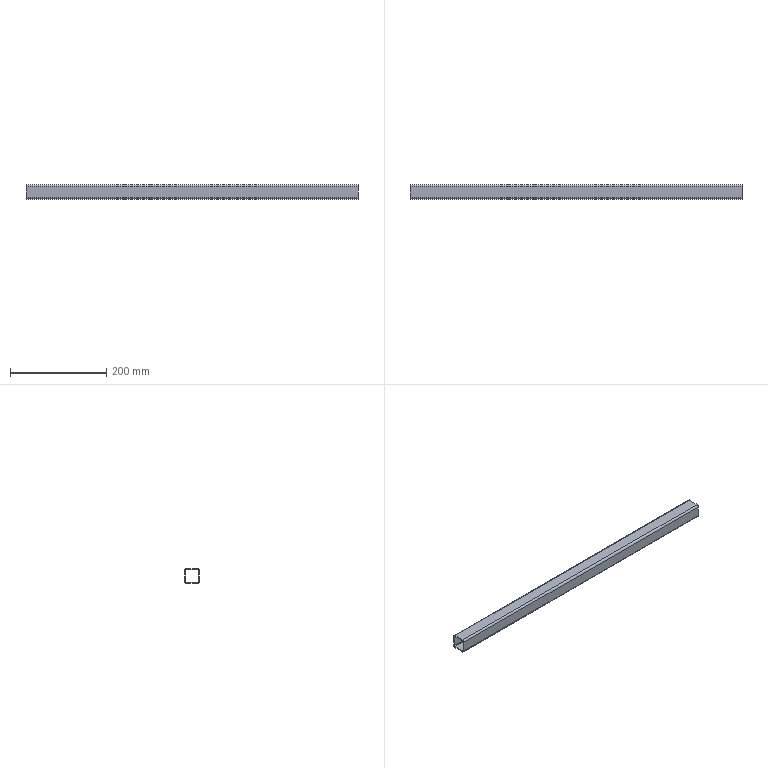Part | SolidWorks | features BaseBody 1, MoveFace 1 | 1 solid | 18 faces | box 690 x 30 x 30 mm | volume 147452 mm3 | plane 10 | cylinder 8 | commonest cylinder face diameters 4 x4 8 x4
STEP:
#1=CARTESIAN_POINT('',(-345.,-776.,31.5));
#2=VERTEX_POINT('',#1);
#3=CARTESIAN_POINT('',(-345.,-780.,27.5));
#4=VERTEX_POINT('',#3);
#5=CARTESIAN_POINT('',(-345.,-776.,27.5));
#6=DIRECTION('',(1.,0.,0.));
#7=DIRECTION('',(0.,0.,-1.));
#8=AXIS2_PLACEMENT_3D('',#5,#6,#7);
#9=CIRCLE('',#8,4.);
#10=EDGE_CURVE('',#2,#4,#9,.T.);
#11=ORIENTED_EDGE('',*,*,#10,.T.);
#12=CARTESIAN_POINT('',(345.,-780.,27.5));
#13=VERTEX_POINT('',#12);
#14=CARTESIAN_POINT('',(373.,-780.,27.5));
#15=DIRECTION('',(-1.,0.,0.));
#16=VECTOR('',#15,1000.);
#17=LINE('',#14,#16);
#18=EDGE_CURVE('',#13,#4,#17,.T.);
#19=ORIENTED_EDGE('',*,*,#18,.F.);
#20=CARTESIAN_POINT('',(345.,-776.,31.5));
#21=VERTEX_POINT('',#20);
#22=CARTESIAN_POINT('',(345.,-776.,27.5));
#23=DIRECTION('',(1.,0.,0.));
#24=DIRECTION('',(0.,0.,-1.));
#25=AXIS2_PLACEMENT_3D('',#22,#23,#24);
#26=CIRCLE('',#25,4.);
#27=EDGE_CURVE('',#21,#13,#26,.T.);
#28=ORIENTED_EDGE('',*,*,#27,.F.);
#29=CARTESIAN_POINT('',(373.,-776.,31.5));
#30=DIRECTION('',(-1.,0.,0.));
#31=VECTOR('',#30,1000.);
#32=LINE('',#29,#31);
#33=EDGE_CURVE('',#21,#2,#32,.T.);
#34=ORIENTED_EDGE('',*,*,#33,.T.);
#35=EDGE_LOOP('',(#11,#19,#28,#34));
#36=FACE_OUTER_BOUND('',#35,.T.);
#37=CARTESIAN_POINT('',(373.,-776.,27.5));
#38=DIRECTION('',(-1.,0.,0.));
#39=DIRECTION('',(0.,0.,1.));
#40=AXIS2_PLACEMENT_3D('',#37,#38,#39);
#41=CYLINDRICAL_SURFACE('',#40,4.);
#42=ADVANCED_FACE('',(#36),#41,.T.);
#43=CARTESIAN_POINT('',(-345.,-780.,5.5));
#44=VERTEX_POINT('',#43);
#45=CARTESIAN_POINT('',(-345.,-780.,27.5));
#46=DIRECTION('',(0.,0.,-1.));
#47=VECTOR('',#46,1000.);
#48=LINE('',#45,#47);
#49=EDGE_CURVE('',#4,#44,#48,.T.);
#50=ORIENTED_EDGE('',*,*,#49,.T.);
#51=CARTESIAN_POINT('',(345.,-780.,5.5));
#52=VERTEX_POINT('',#51);
#53=CARTESIAN_POINT('',(373.,-780.,5.5));
#54=DIRECTION('',(-1.,0.,0.));
#55=VECTOR('',#54,1000.);
#56=LINE('',#53,#55);
#57=EDGE_CURVE('',#52,#44,#56,.T.);
#58=ORIENTED_EDGE('',*,*,#57,.F.);
#59=CARTESIAN_POINT('',(345.,-780.,27.5));
#60=DIRECTION('',(0.,0.,-1.));
#61=VECTOR('',#60,1000.);
#62=LINE('',#59,#61);
#63=EDGE_CURVE('',#13,#52,#62,.T.);
#64=ORIENTED_EDGE('',*,*,#63,.F.);
#65=ORIENTED_EDGE('',*,*,#18,.T.);
#66=EDGE_LOOP('',(#50,#58,#64,#65));
#67=FACE_OUTER_BOUND('',#66,.T.);
#68=CARTESIAN_POINT('',(373.,-780.,27.5));
#69=DIRECTION('',(0.,1.,0.));
#70=DIRECTION('',(0.,0.,1.));
#71=AXIS2_PLACEMENT_3D('',#68,#69,#70);
#72=PLANE('',#71);
#73=ADVANCED_FACE('',(#67),#72,.F.);
#74=CARTESIAN_POINT('',(-345.,-776.,1.5));
#75=VERTEX_POINT('',#74);
#76=CARTESIAN_POINT('',(-345.,-776.,5.5));
#77=DIRECTION('',(1.,0.,0.));
#78=DIRECTION('',(0.,0.,-1.));
#79=AXIS2_PLACEMENT_3D('',#76,#77,#78);
#80=CIRCLE('',#79,4.);
#81=EDGE_CURVE('',#44,#75,#80,.T.);
#82=ORIENTED_EDGE('',*,*,#81,.T.);
#83=CARTESIAN_POINT('',(345.,-776.,1.5));
#84=VERTEX_POINT('',#83);
#85=CARTESIAN_POINT('',(373.,-776.,1.5));
#86=DIRECTION('',(-1.,0.,0.));
#87=VECTOR('',#86,1000.);
#88=LINE('',#85,#87);
#89=EDGE_CURVE('',#84,#75,#88,.T.);
#90=ORIENTED_EDGE('',*,*,#89,.F.);
#91=CARTESIAN_POINT('',(345.,-776.,5.5));
#92=DIRECTION('',(1.,0.,0.));
#93=DIRECTION('',(0.,0.,-1.));
#94=AXIS2_PLACEMENT_3D('',#91,#92,#93);
#95=CIRCLE('',#94,4.);
#96=EDGE_CURVE('',#52,#84,#95,.T.);
#97=ORIENTED_EDGE('',*,*,#96,.F.);
#98=ORIENTED_EDGE('',*,*,#57,.T.);
#99=EDGE_LOOP('',(#82,#90,#97,#98));
#100=FACE_OUTER_BOUND('',#99,.T.);
#101=CARTESIAN_POINT('',(373.,-776.,5.5));
#102=DIRECTION('',(-1.,0.,0.));
#103=DIRECTION('',(0.,0.,1.));
#104=AXIS2_PLACEMENT_3D('',#101,#102,#103);
#105=CYLINDRICAL_SURFACE('',#104,4.);
#106=ADVANCED_FACE('',(#100),#105,.T.);
#107=CARTESIAN_POINT('',(-345.,-754.,1.5));
#108=VERTEX_POINT('',#107);
#109=CARTESIAN_POINT('',(-345.,-754.,1.5));
#110=DIRECTION('',(0.,1.,0.));
#111=VECTOR('',#110,1000.);
#112=LINE('',#109,#111);
#113=EDGE_CURVE('',#75,#108,#112,.T.);
#114=ORIENTED_EDGE('',*,*,#113,.T.);
#115=CARTESIAN_POINT('',(345.,-754.,1.5));
#116=VERTEX_POINT('',#115);
#117=CARTESIAN_POINT('',(373.,-754.,1.5));
#118=DIRECTION('',(-1.,0.,0.));
#119=VECTOR('',#118,1000.);
#120=LINE('',#117,#119);
#121=EDGE_CURVE('',#116,#108,#120,.T.);
#122=ORIENTED_EDGE('',*,*,#121,.F.);
#123=CARTESIAN_POINT('',(345.,-754.,1.5));
#124=DIRECTION('',(0.,1.,0.));
#125=VECTOR('',#124,1000.);
#126=LINE('',#123,#125);
#127=EDGE_CURVE('',#84,#116,#126,.T.);
#128=ORIENTED_EDGE('',*,*,#127,.F.);
#129=ORIENTED_EDGE('',*,*,#89,.T.);
#130=EDGE_LOOP('',(#114,#122,#128,#129));
#131=FACE_OUTER_BOUND('',#130,.T.);
#132=CARTESIAN_POINT('',(373.,-754.,1.5));
#133=DIRECTION('',(0.,0.,1.));
#134=DIRECTION('',(1.,0.,0.));
#135=AXIS2_PLACEMENT_3D('',#132,#133,#134);
#136=PLANE('',#135);
#137=ADVANCED_FACE('',(#131),#136,.F.);
#138=CARTESIAN_POINT('',(-345.,-750.,5.5));
#139=VERTEX_POINT('',#138);
#140=CARTESIAN_POINT('',(-345.,-754.,5.5));
#141=DIRECTION('',(1.,0.,0.));
#142=DIRECTION('',(0.,0.,-1.));
#143=AXIS2_PLACEMENT_3D('',#140,#141,#142);
#144=CIRCLE('',#143,4.);
#145=EDGE_CURVE('',#108,#139,#144,.T.);
#146=ORIENTED_EDGE('',*,*,#145,.T.);
#147=CARTESIAN_POINT('',(345.,-750.,5.5));
#148=VERTEX_POINT('',#147);
#149=CARTESIAN_POINT('',(373.,-750.,5.5));
#150=DIRECTION('',(-1.,0.,0.));
#151=VECTOR('',#150,1000.);
#152=LINE('',#149,#151);
#153=EDGE_CURVE('',#148,#139,#152,.T.);
#154=ORIENTED_EDGE('',*,*,#153,.F.);
#155=CARTESIAN_POINT('',(345.,-754.,5.5));
#156=DIRECTION('',(1.,0.,0.));
#157=DIRECTION('',(0.,0.,-1.));
#158=AXIS2_PLACEMENT_3D('',#155,#156,#157);
#159=CIRCLE('',#158,4.);
#160=EDGE_CURVE('',#116,#148,#159,.T.);
#161=ORIENTED_EDGE('',*,*,#160,.F.);
#162=ORIENTED_EDGE('',*,*,#121,.T.);
#163=EDGE_LOOP('',(#146,#154,#161,#162));
#164=FACE_OUTER_BOUND('',#163,.T.);
#165=CARTESIAN_POINT('',(373.,-754.,5.5));
#166=DIRECTION('',(-1.,0.,0.));
#167=DIRECTION('',(0.,0.,1.));
#168=AXIS2_PLACEMENT_3D('',#165,#166,#167);
#169=CYLINDRICAL_SURFACE('',#168,4.);
#170=ADVANCED_FACE('',(#164),#169,.T.);
#171=CARTESIAN_POINT('',(-345.,-750.,27.5));
#172=VERTEX_POINT('',#171);
#173=CARTESIAN_POINT('',(-345.,-750.,5.5));
#174=DIRECTION('',(0.,0.,1.));
#175=VECTOR('',#174,1000.);
#176=LINE('',#173,#175);
#177=EDGE_CURVE('',#139,#172,#176,.T.);
#178=ORIENTED_EDGE('',*,*,#177,.T.);
#179=CARTESIAN_POINT('',(345.,-750.,27.5));
#180=VERTEX_POINT('',#179);
#181=CARTESIAN_POINT('',(373.,-750.,27.5));
#182=DIRECTION('',(-1.,0.,0.));
#183=VECTOR('',#182,1000.);
#184=LINE('',#181,#183);
#185=EDGE_CURVE('',#180,#172,#184,.T.);
#186=ORIENTED_EDGE('',*,*,#185,.F.);
#187=CARTESIAN_POINT('',(345.,-750.,5.5));
#188=DIRECTION('',(0.,0.,1.));
#189=VECTOR('',#188,1000.);
#190=LINE('',#187,#189);
#191=EDGE_CURVE('',#148,#180,#190,.T.);
#192=ORIENTED_EDGE('',*,*,#191,.F.);
#193=ORIENTED_EDGE('',*,*,#153,.T.);
#194=EDGE_LOOP('',(#178,#186,#192,#193));
#195=FACE_OUTER_BOUND('',#194,.T.);
#196=CARTESIAN_POINT('',(373.,-750.,5.5));
#197=DIRECTION('',(0.,-1.,0.));
#198=DIRECTION('',(0.,0.,-1.));
#199=AXIS2_PLACEMENT_3D('',#196,#197,#198);
#200=PLANE('',#199);
#201=ADVANCED_FACE('',(#195),#200,.F.);
#202=CARTESIAN_POINT('',(-345.,-754.,31.5));
#203=VERTEX_POINT('',#202);
#204=CARTESIAN_POINT('',(-345.,-754.,27.5));
#205=DIRECTION('',(1.,0.,0.));
#206=DIRECTION('',(0.,0.,-1.));
#207=AXIS2_PLACEMENT_3D('',#204,#205,#206);
#208=CIRCLE('',#207,4.);
#209=EDGE_CURVE('',#172,#203,#208,.T.);
#210=ORIENTED_EDGE('',*,*,#209,.T.);
#211=CARTESIAN_POINT('',(345.,-754.,31.5));
#212=VERTEX_POINT('',#211);
#213=CARTESIAN_POINT('',(373.,-754.,31.5));
#214=DIRECTION('',(-1.,0.,0.));
#215=VECTOR('',#214,1000.);
#216=LINE('',#213,#215);
#217=EDGE_CURVE('',#212,#203,#216,.T.);
#218=ORIENTED_EDGE('',*,*,#217,.F.);
#219=CARTESIAN_POINT('',(345.,-754.,27.5));
#220=DIRECTION('',(1.,0.,0.));
#221=DIRECTION('',(0.,0.,-1.));
#222=AXIS2_PLACEMENT_3D('',#219,#220,#221);
#223=CIRCLE('',#222,4.);
#224=EDGE_CURVE('',#180,#212,#223,.T.);
#225=ORIENTED_EDGE('',*,*,#224,.F.);
#226=ORIENTED_EDGE('',*,*,#185,.T.);
#227=EDGE_LOOP('',(#210,#218,#225,#226));
#228=FACE_OUTER_BOUND('',#227,.T.);
#229=CARTESIAN_POINT('',(373.,-754.,27.5));
#230=DIRECTION('',(-1.,0.,0.));
#231=DIRECTION('',(0.,0.,1.));
#232=AXIS2_PLACEMENT_3D('',#229,#230,#231);
#233=CYLINDRICAL_SURFACE('',#232,4.);
#234=ADVANCED_FACE('',(#228),#233,.T.);
#235=CARTESIAN_POINT('',(-345.,-778.,5.5));
#236=VERTEX_POINT('',#235);
#237=CARTESIAN_POINT('',(-345.,-776.,3.5));
#238=VERTEX_POINT('',#237);
#239=CARTESIAN_POINT('',(-345.,-776.,5.5));
#240=DIRECTION('',(1.,0.,0.));
#241=DIRECTION('',(0.,0.,-1.));
#242=AXIS2_PLACEMENT_3D('',#239,#240,#241);
#243=CIRCLE('',#242,2.);
#244=EDGE_CURVE('',#236,#238,#243,.T.);
#245=ORIENTED_EDGE('',*,*,#244,.F.);
#246=CARTESIAN_POINT('',(345.,-778.,5.5));
#247=VERTEX_POINT('',#246);
#248=CARTESIAN_POINT('',(373.,-778.,5.5));
#249=DIRECTION('',(-1.,0.,0.));
#250=VECTOR('',#249,1000.);
#251=LINE('',#248,#250);
#252=EDGE_CURVE('',#247,#236,#251,.T.);
#253=ORIENTED_EDGE('',*,*,#252,.F.);
#254=CARTESIAN_POINT('',(345.,-776.,3.5));
#255=VERTEX_POINT('',#254);
#256=CARTESIAN_POINT('',(345.,-776.,5.5));
#257=DIRECTION('',(1.,0.,0.));
#258=DIRECTION('',(0.,0.,-1.));
#259=AXIS2_PLACEMENT_3D('',#256,#257,#258);
#260=CIRCLE('',#259,2.);
#261=EDGE_CURVE('',#247,#255,#260,.T.);
#262=ORIENTED_EDGE('',*,*,#261,.T.);
#263=CARTESIAN_POINT('',(373.,-776.,3.5));
#264=DIRECTION('',(-1.,0.,0.));
#265=VECTOR('',#264,1000.);
#266=LINE('',#263,#265);
#267=EDGE_CURVE('',#255,#238,#266,.T.);
#268=ORIENTED_EDGE('',*,*,#267,.T.);
#269=EDGE_LOOP('',(#245,#253,#262,#268));
#270=FACE_OUTER_BOUND('',#269,.T.);
#271=CARTESIAN_POINT('',(373.,-776.,5.5));
#272=DIRECTION('',(-1.,0.,0.));
#273=DIRECTION('',(0.,0.,1.));
#274=AXIS2_PLACEMENT_3D('',#271,#272,#273);
#275=CYLINDRICAL_SURFACE('',#274,2.);
#276=ADVANCED_FACE('',(#270),#275,.F.);
#277=CARTESIAN_POINT('',(-345.,-778.,27.5));
#278=VERTEX_POINT('',#277);
#279=CARTESIAN_POINT('',(-345.,-778.,27.5));
#280=DIRECTION('',(0.,0.,-1.));
#281=VECTOR('',#280,1000.);
#282=LINE('',#279,#281);
#283=EDGE_CURVE('',#278,#236,#282,.T.);
#284=ORIENTED_EDGE('',*,*,#283,.F.);
#285=CARTESIAN_POINT('',(345.,-778.,27.5));
#286=VERTEX_POINT('',#285);
#287=CARTESIAN_POINT('',(373.,-778.,27.5));
#288=DIRECTION('',(-1.,0.,0.));
#289=VECTOR('',#288,1000.);
#290=LINE('',#287,#289);
#291=EDGE_CURVE('',#286,#278,#290,.T.);
#292=ORIENTED_EDGE('',*,*,#291,.F.);
#293=CARTESIAN_POINT('',(345.,-778.,27.5));
#294=DIRECTION('',(0.,0.,-1.));
#295=VECTOR('',#294,1000.);
#296=LINE('',#293,#295);
#297=EDGE_CURVE('',#286,#247,#296,.T.);
#298=ORIENTED_EDGE('',*,*,#297,.T.);
#299=ORIENTED_EDGE('',*,*,#252,.T.);
#300=EDGE_LOOP('',(#284,#292,#298,#299));
#301=FACE_OUTER_BOUND('',#300,.T.);
#302=CARTESIAN_POINT('',(373.,-778.,27.5));
#303=DIRECTION('',(0.,1.,0.));
#304=DIRECTION('',(0.,0.,1.));
#305=AXIS2_PLACEMENT_3D('',#302,#303,#304);
#306=PLANE('',#305);
#307=ADVANCED_FACE('',(#301),#306,.T.);
#308=CARTESIAN_POINT('',(-345.,-776.,29.5));
#309=VERTEX_POINT('',#308);
#310=CARTESIAN_POINT('',(-345.,-776.,27.5));
#311=DIRECTION('',(1.,0.,0.));
#312=DIRECTION('',(0.,0.,-1.));
#313=AXIS2_PLACEMENT_3D('',#310,#311,#312);
#314=CIRCLE('',#313,2.);
#315=EDGE_CURVE('',#309,#278,#314,.T.);
#316=ORIENTED_EDGE('',*,*,#315,.F.);
#317=CARTESIAN_POINT('',(345.,-776.,29.5));
#318=VERTEX_POINT('',#317);
#319=CARTESIAN_POINT('',(373.,-776.,29.5));
#320=DIRECTION('',(-1.,0.,0.));
#321=VECTOR('',#320,1000.);
#322=LINE('',#319,#321);
#323=EDGE_CURVE('',#318,#309,#322,.T.);
#324=ORIENTED_EDGE('',*,*,#323,.F.);
#325=CARTESIAN_POINT('',(345.,-776.,27.5));
#326=DIRECTION('',(1.,0.,0.));
#327=DIRECTION('',(0.,0.,-1.));
#328=AXIS2_PLACEMENT_3D('',#325,#326,#327);
#329=CIRCLE('',#328,2.);
#330=EDGE_CURVE('',#318,#286,#329,.T.);
#331=ORIENTED_EDGE('',*,*,#330,.T.);
#332=ORIENTED_EDGE('',*,*,#291,.T.);
#333=EDGE_LOOP('',(#316,#324,#331,#332));
#334=FACE_OUTER_BOUND('',#333,.T.);
#335=CARTESIAN_POINT('',(373.,-776.,27.5));
#336=DIRECTION('',(-1.,0.,0.));
#337=DIRECTION('',(0.,0.,1.));
#338=AXIS2_PLACEMENT_3D('',#335,#336,#337);
#339=CYLINDRICAL_SURFACE('',#338,2.);
#340=ADVANCED_FACE('',(#334),#339,.F.);
#341=CARTESIAN_POINT('',(-345.,-754.,29.5));
#342=VERTEX_POINT('',#341);
#343=CARTESIAN_POINT('',(-345.,-776.,29.5));
#344=DIRECTION('',(0.,-1.,0.));
#345=VECTOR('',#344,1000.);
#346=LINE('',#343,#345);
#347=EDGE_CURVE('',#342,#309,#346,.T.);
#348=ORIENTED_EDGE('',*,*,#347,.F.);
#349=CARTESIAN_POINT('',(345.,-754.,29.5));
#350=VERTEX_POINT('',#349);
#351=CARTESIAN_POINT('',(373.,-754.,29.5));
#352=DIRECTION('',(-1.,0.,0.));
#353=VECTOR('',#352,1000.);
#354=LINE('',#351,#353);
#355=EDGE_CURVE('',#350,#342,#354,.T.);
#356=ORIENTED_EDGE('',*,*,#355,.F.);
#357=CARTESIAN_POINT('',(345.,-776.,29.5));
#358=DIRECTION('',(0.,-1.,0.));
#359=VECTOR('',#358,1000.);
#360=LINE('',#357,#359);
#361=EDGE_CURVE('',#350,#318,#360,.T.);
#362=ORIENTED_EDGE('',*,*,#361,.T.);
#363=ORIENTED_EDGE('',*,*,#323,.T.);
#364=EDGE_LOOP('',(#348,#356,#362,#363));
#365=FACE_OUTER_BOUND('',#364,.T.);
#366=CARTESIAN_POINT('',(373.,-776.,29.5));
#367=DIRECTION('',(0.,0.,-1.));
#368=DIRECTION('',(-1.,0.,0.));
#369=AXIS2_PLACEMENT_3D('',#366,#367,#368);
#370=PLANE('',#369);
#371=ADVANCED_FACE('',(#365),#370,.T.);
#372=CARTESIAN_POINT('',(-345.,-752.,27.5));
#373=VERTEX_POINT('',#372);
#374=CARTESIAN_POINT('',(-345.,-754.,27.5));
#375=DIRECTION('',(1.,0.,0.));
#376=DIRECTION('',(0.,0.,-1.));
#377=AXIS2_PLACEMENT_3D('',#374,#375,#376);
#378=CIRCLE('',#377,2.);
#379=EDGE_CURVE('',#373,#342,#378,.T.);
#380=ORIENTED_EDGE('',*,*,#379,.F.);
#381=CARTESIAN_POINT('',(345.,-752.,27.5));
#382=VERTEX_POINT('',#381);
#383=CARTESIAN_POINT('',(373.,-752.,27.5));
#384=DIRECTION('',(-1.,0.,0.));
#385=VECTOR('',#384,1000.);
#386=LINE('',#383,#385);
#387=EDGE_CURVE('',#382,#373,#386,.T.);
#388=ORIENTED_EDGE('',*,*,#387,.F.);
#389=CARTESIAN_POINT('',(345.,-754.,27.5));
#390=DIRECTION('',(1.,0.,0.));
#391=DIRECTION('',(0.,0.,-1.));
#392=AXIS2_PLACEMENT_3D('',#389,#390,#391);
#393=CIRCLE('',#392,2.);
#394=EDGE_CURVE('',#382,#350,#393,.T.);
#395=ORIENTED_EDGE('',*,*,#394,.T.);
#396=ORIENTED_EDGE('',*,*,#355,.T.);
#397=EDGE_LOOP('',(#380,#388,#395,#396));
#398=FACE_OUTER_BOUND('',#397,.T.);
#399=CARTESIAN_POINT('',(373.,-754.,27.5));
#400=DIRECTION('',(-1.,0.,0.));
#401=DIRECTION('',(0.,0.,1.));
#402=AXIS2_PLACEMENT_3D('',#399,#400,#401);
#403=CYLINDRICAL_SURFACE('',#402,2.);
#404=ADVANCED_FACE('',(#398),#403,.F.);
#405=CARTESIAN_POINT('',(-345.,-752.,5.5));
#406=VERTEX_POINT('',#405);
#407=CARTESIAN_POINT('',(-345.,-752.,5.5));
#408=DIRECTION('',(0.,0.,1.));
#409=VECTOR('',#408,1000.);
#410=LINE('',#407,#409);
#411=EDGE_CURVE('',#406,#373,#410,.T.);
#412=ORIENTED_EDGE('',*,*,#411,.F.);
#413=CARTESIAN_POINT('',(345.,-752.,5.5));
#414=VERTEX_POINT('',#413);
#415=CARTESIAN_POINT('',(373.,-752.,5.5));
#416=DIRECTION('',(-1.,0.,0.));
#417=VECTOR('',#416,1000.);
#418=LINE('',#415,#417);
#419=EDGE_CURVE('',#414,#406,#418,.T.);
#420=ORIENTED_EDGE('',*,*,#419,.F.);
#421=CARTESIAN_POINT('',(345.,-752.,5.5));
#422=DIRECTION('',(0.,0.,1.));
#423=VECTOR('',#422,1000.);
#424=LINE('',#421,#423);
#425=EDGE_CURVE('',#414,#382,#424,.T.);
#426=ORIENTED_EDGE('',*,*,#425,.T.);
#427=ORIENTED_EDGE('',*,*,#387,.T.);
#428=EDGE_LOOP('',(#412,#420,#426,#427));
#429=FACE_OUTER_BOUND('',#428,.T.);
#430=CARTESIAN_POINT('',(373.,-752.,5.5));
#431=DIRECTION('',(0.,-1.,0.));
#432=DIRECTION('',(0.,0.,-1.));
#433=AXIS2_PLACEMENT_3D('',#430,#431,#432);
#434=PLANE('',#433);
#435=ADVANCED_FACE('',(#429),#434,.T.);
#436=CARTESIAN_POINT('',(-345.,-754.,3.5));
#437=VERTEX_POINT('',#436);
#438=CARTESIAN_POINT('',(-345.,-754.,5.5));
#439=DIRECTION('',(1.,0.,0.));
#440=DIRECTION('',(0.,0.,-1.));
#441=AXIS2_PLACEMENT_3D('',#438,#439,#440);
#442=CIRCLE('',#441,2.);
#443=EDGE_CURVE('',#437,#406,#442,.T.);
#444=ORIENTED_EDGE('',*,*,#443,.F.);
#445=CARTESIAN_POINT('',(345.,-754.,3.5));
#446=VERTEX_POINT('',#445);
#447=CARTESIAN_POINT('',(373.,-754.,3.5));
#448=DIRECTION('',(-1.,0.,0.));
#449=VECTOR('',#448,1000.);
#450=LINE('',#447,#449);
#451=EDGE_CURVE('',#446,#437,#450,.T.);
#452=ORIENTED_EDGE('',*,*,#451,.F.);
#453=CARTESIAN_POINT('',(345.,-754.,5.5));
#454=DIRECTION('',(1.,0.,0.));
#455=DIRECTION('',(0.,0.,-1.));
#456=AXIS2_PLACEMENT_3D('',#453,#454,#455);
#457=CIRCLE('',#456,2.);
#458=EDGE_CURVE('',#446,#414,#457,.T.);
#459=ORIENTED_EDGE('',*,*,#458,.T.);
#460=ORIENTED_EDGE('',*,*,#419,.T.);
#461=EDGE_LOOP('',(#444,#452,#459,#460));
#462=FACE_OUTER_BOUND('',#461,.T.);
#463=CARTESIAN_POINT('',(373.,-754.,5.5));
#464=DIRECTION('',(-1.,0.,0.));
#465=DIRECTION('',(0.,0.,1.));
#466=AXIS2_PLACEMENT_3D('',#463,#464,#465);
#467=CYLINDRICAL_SURFACE('',#466,2.);
#468=ADVANCED_FACE('',(#462),#467,.F.);
#469=CARTESIAN_POINT('',(-345.,-754.,3.5));
#470=DIRECTION('',(0.,1.,0.));
#471=VECTOR('',#470,1000.);
#472=LINE('',#469,#471);
#473=EDGE_CURVE('',#238,#437,#472,.T.);
#474=ORIENTED_EDGE('',*,*,#473,.F.);
#475=ORIENTED_EDGE('',*,*,#267,.F.);
#476=CARTESIAN_POINT('',(345.,-754.,3.5));
#477=DIRECTION('',(0.,1.,0.));
#478=VECTOR('',#477,1000.);
#479=LINE('',#476,#478);
#480=EDGE_CURVE('',#255,#446,#479,.T.);
#481=ORIENTED_EDGE('',*,*,#480,.T.);
#482=ORIENTED_EDGE('',*,*,#451,.T.);
#483=EDGE_LOOP('',(#474,#475,#481,#482));
#484=FACE_OUTER_BOUND('',#483,.T.);
#485=CARTESIAN_POINT('',(373.,-754.,3.5));
#486=DIRECTION('',(0.,0.,1.));
#487=DIRECTION('',(1.,0.,0.));
#488=AXIS2_PLACEMENT_3D('',#485,#486,#487);
#489=PLANE('',#488);
#490=ADVANCED_FACE('',(#484),#489,.T.);
#491=CARTESIAN_POINT('',(-345.,-776.,31.5));
#492=DIRECTION('',(0.,-1.,0.));
#493=VECTOR('',#492,1000.);
#494=LINE('',#491,#493);
#495=EDGE_CURVE('',#203,#2,#494,.T.);
#496=ORIENTED_EDGE('',*,*,#495,.T.);
#497=ORIENTED_EDGE('',*,*,#33,.F.);
#498=CARTESIAN_POINT('',(345.,-776.,31.5));
#499=DIRECTION('',(0.,-1.,0.));
#500=VECTOR('',#499,1000.);
#501=LINE('',#498,#500);
#502=EDGE_CURVE('',#212,#21,#501,.T.);
#503=ORIENTED_EDGE('',*,*,#502,.F.);
#504=ORIENTED_EDGE('',*,*,#217,.T.);
#505=EDGE_LOOP('',(#496,#497,#503,#504));
#506=FACE_OUTER_BOUND('',#505,.T.);
#507=CARTESIAN_POINT('',(373.,-776.,31.5));
#508=DIRECTION('',(0.,0.,-1.));
#509=DIRECTION('',(-1.,0.,0.));
#510=AXIS2_PLACEMENT_3D('',#507,#508,#509);
#511=PLANE('',#510);
#512=ADVANCED_FACE('',(#506),#511,.F.);
#513=ORIENTED_EDGE('',*,*,#261,.F.);
#514=ORIENTED_EDGE('',*,*,#297,.F.);
#515=ORIENTED_EDGE('',*,*,#330,.F.);
#516=ORIENTED_EDGE('',*,*,#361,.F.);
#517=ORIENTED_EDGE('',*,*,#394,.F.);
#518=ORIENTED_EDGE('',*,*,#425,.F.);
#519=ORIENTED_EDGE('',*,*,#458,.F.);
#520=ORIENTED_EDGE('',*,*,#480,.F.);
#521=EDGE_LOOP('',(#513,#514,#515,#516,#517,#518,#519,#520));
#522=FACE_BOUND('',#521,.T.);
#523=ORIENTED_EDGE('',*,*,#27,.T.);
#524=ORIENTED_EDGE('',*,*,#63,.T.);
#525=ORIENTED_EDGE('',*,*,#96,.T.);
#526=ORIENTED_EDGE('',*,*,#127,.T.);
#527=ORIENTED_EDGE('',*,*,#160,.T.);
#528=ORIENTED_EDGE('',*,*,#191,.T.);
#529=ORIENTED_EDGE('',*,*,#224,.T.);
#530=ORIENTED_EDGE('',*,*,#502,.T.);
#531=EDGE_LOOP('',(#523,#524,#525,#526,#527,#528,#529,#530));
#532=FACE_OUTER_BOUND('',#531,.T.);
#533=CARTESIAN_POINT('',(345.,-776.,27.5));
#534=DIRECTION('',(1.,0.,0.));
#535=DIRECTION('',(0.,0.,-1.));
#536=AXIS2_PLACEMENT_3D('',#533,#534,#535);
#537=PLANE('',#536);
#538=ADVANCED_FACE('',(#522,#532),#537,.T.);
#539=ORIENTED_EDGE('',*,*,#244,.T.);
#540=ORIENTED_EDGE('',*,*,#473,.T.);
#541=ORIENTED_EDGE('',*,*,#443,.T.);
#542=ORIENTED_EDGE('',*,*,#411,.T.);
#543=ORIENTED_EDGE('',*,*,#379,.T.);
#544=ORIENTED_EDGE('',*,*,#347,.T.);
#545=ORIENTED_EDGE('',*,*,#315,.T.);
#546=ORIENTED_EDGE('',*,*,#283,.T.);
#547=EDGE_LOOP('',(#539,#540,#541,#542,#543,#544,#545,#546));
#548=FACE_BOUND('',#547,.T.);
#549=ORIENTED_EDGE('',*,*,#10,.F.);
#550=ORIENTED_EDGE('',*,*,#495,.F.);
#551=ORIENTED_EDGE('',*,*,#209,.F.);
#552=ORIENTED_EDGE('',*,*,#177,.F.);
#553=ORIENTED_EDGE('',*,*,#145,.F.);
#554=ORIENTED_EDGE('',*,*,#113,.F.);
#555=ORIENTED_EDGE('',*,*,#81,.F.);
#556=ORIENTED_EDGE('',*,*,#49,.F.);
#557=EDGE_LOOP('',(#549,#550,#551,#552,#553,#554,#555,#556));
#558=FACE_OUTER_BOUND('',#557,.T.);
#559=CARTESIAN_POINT('',(-345.,-776.,27.5));
#560=DIRECTION('',(1.,0.,0.));
#561=DIRECTION('',(0.,0.,-1.));
#562=AXIS2_PLACEMENT_3D('',#559,#560,#561);
#563=PLANE('',#562);
#564=ADVANCED_FACE('',(#548,#558),#563,.F.);
#565=CLOSED_SHELL('',(#42,#73,#106,#137,#170,#201,#234,#276,#307,#340,#371,#404,#435,#468,#490,#512,#538,#564));
#566=MANIFOLD_SOLID_BREP('',#565);
#567=CARTESIAN_POINT('',(0.,0.,0.));
#568=DIRECTION('',(0.,0.,1.));
#569=DIRECTION('',(1.,0.,0.));
#570=AXIS2_PLACEMENT_3D('',#567,#568,#569);
#571=(LENGTH_UNIT()NAMED_UNIT(*)SI_UNIT(.MILLI.,.METRE.));
#572=UNCERTAINTY_MEASURE_WITH_UNIT(LENGTH_MEASURE(0.00001),#571,'','');
#573=(NAMED_UNIT(*)PLANE_ANGLE_UNIT()SI_UNIT($,.RADIAN.));
#574=(NAMED_UNIT(*)SI_UNIT($,.STERADIAN.)SOLID_ANGLE_UNIT());
#575=(GEOMETRIC_REPRESENTATION_CONTEXT(3)GLOBAL_UNCERTAINTY_ASSIGNED_CONTEXT((#572))GLOBAL_UNIT_ASSIGNED_CONTEXT((#571,#573,#574))REPRESENTATION_CONTEXT('',''));
#576=ADVANCED_BREP_SHAPE_REPRESENTATION('',(#566,#570),#575);